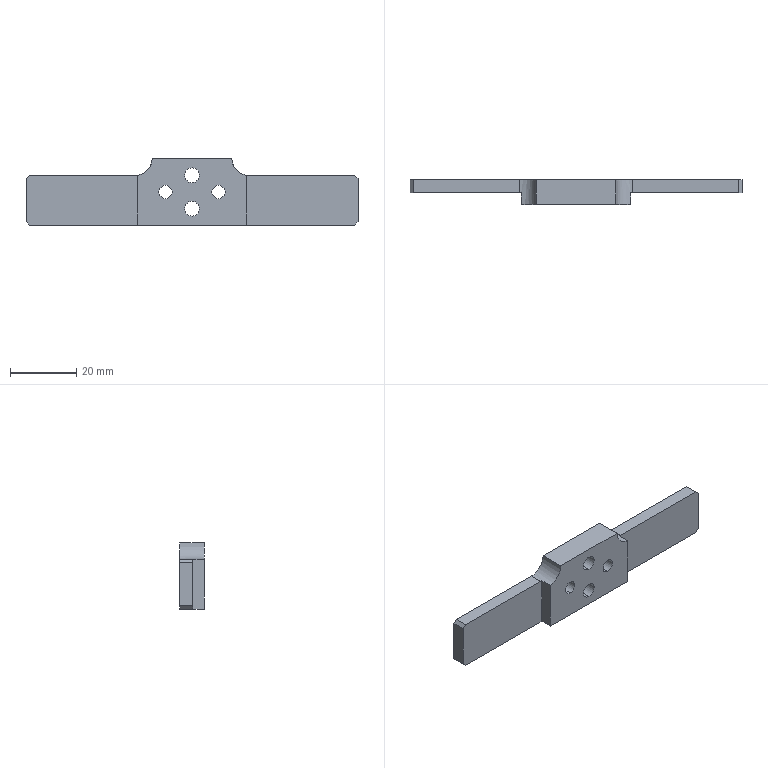Part | SolidWorks | features ICE 6, Chamfer 2, LPattern 2, Cut 1, Extrusion 1, Fillet 1, HoleWzd 1 | 1 solid | 26 faces | box 100 x 7.5 x 20 mm | volume 8278 mm3 | plane 16 | cylinder 10 | commonest cylinder face diameters 4 x4 4.5 x4 10 x2
STEP:
#1=CARTESIAN_POINT('',(-62.,-5.5,-7.));
#2=VERTEX_POINT('',#1);
#3=CARTESIAN_POINT('',(-62.,-5.5,-3.));
#4=VERTEX_POINT('',#3);
#5=CARTESIAN_POINT('',(-62.,-5.5,-5.));
#6=DIRECTION('',(0.,1.,0.));
#7=DIRECTION('',(0.,0.,1.));
#8=AXIS2_PLACEMENT_3D('',#5,#6,#7);
#9=CIRCLE('',#8,2.);
#10=EDGE_CURVE('',#2,#4,#9,.T.);
#11=ORIENTED_EDGE('',*,*,#10,.F.);
#12=CARTESIAN_POINT('',(-62.,2.,-7.));
#13=VERTEX_POINT('',#12);
#14=CARTESIAN_POINT('',(-62.,2.,-7.));
#15=DIRECTION('',(0.,1.,0.));
#16=VECTOR('',#15,1000.);
#17=LINE('',#14,#16);
#18=EDGE_CURVE('',#2,#13,#17,.T.);
#19=ORIENTED_EDGE('',*,*,#18,.T.);
#20=CARTESIAN_POINT('',(-62.,2.,-3.));
#21=VERTEX_POINT('',#20);
#22=CARTESIAN_POINT('',(-62.,2.,-5.));
#23=DIRECTION('',(0.,1.,0.));
#24=DIRECTION('',(0.,0.,1.));
#25=AXIS2_PLACEMENT_3D('',#22,#23,#24);
#26=CIRCLE('',#25,2.);
#27=EDGE_CURVE('',#13,#21,#26,.T.);
#28=ORIENTED_EDGE('',*,*,#27,.T.);
#29=CARTESIAN_POINT('',(-62.,2.,-3.));
#30=DIRECTION('',(0.,1.,0.));
#31=VECTOR('',#30,1000.);
#32=LINE('',#29,#31);
#33=EDGE_CURVE('',#4,#21,#32,.T.);
#34=ORIENTED_EDGE('',*,*,#33,.F.);
#35=EDGE_LOOP('',(#11,#19,#28,#34));
#36=FACE_OUTER_BOUND('',#35,.T.);
#37=CARTESIAN_POINT('',(-62.,2.,-5.));
#38=DIRECTION('',(0.,1.,0.));
#39=DIRECTION('',(0.,0.,1.));
#40=AXIS2_PLACEMENT_3D('',#37,#38,#39);
#41=CYLINDRICAL_SURFACE('',#40,2.);
#42=ADVANCED_FACE('',(#36),#41,.F.);
#43=CARTESIAN_POINT('',(-78.,-5.5,-7.));
#44=VERTEX_POINT('',#43);
#45=CARTESIAN_POINT('',(-78.,-5.5,-3.));
#46=VERTEX_POINT('',#45);
#47=CARTESIAN_POINT('',(-78.,-5.5,-5.));
#48=DIRECTION('',(0.,1.,0.));
#49=DIRECTION('',(0.,0.,1.));
#50=AXIS2_PLACEMENT_3D('',#47,#48,#49);
#51=CIRCLE('',#50,2.);
#52=EDGE_CURVE('',#44,#46,#51,.T.);
#53=ORIENTED_EDGE('',*,*,#52,.F.);
#54=CARTESIAN_POINT('',(-78.,2.,-7.));
#55=VERTEX_POINT('',#54);
#56=CARTESIAN_POINT('',(-78.,2.,-7.));
#57=DIRECTION('',(0.,1.,0.));
#58=VECTOR('',#57,1000.);
#59=LINE('',#56,#58);
#60=EDGE_CURVE('',#44,#55,#59,.T.);
#61=ORIENTED_EDGE('',*,*,#60,.T.);
#62=CARTESIAN_POINT('',(-78.,2.,-3.));
#63=VERTEX_POINT('',#62);
#64=CARTESIAN_POINT('',(-78.,2.,-5.));
#65=DIRECTION('',(0.,1.,0.));
#66=DIRECTION('',(0.,0.,1.));
#67=AXIS2_PLACEMENT_3D('',#64,#65,#66);
#68=CIRCLE('',#67,2.);
#69=EDGE_CURVE('',#55,#63,#68,.T.);
#70=ORIENTED_EDGE('',*,*,#69,.T.);
#71=CARTESIAN_POINT('',(-78.,2.,-3.));
#72=DIRECTION('',(0.,1.,0.));
#73=VECTOR('',#72,1000.);
#74=LINE('',#71,#73);
#75=EDGE_CURVE('',#46,#63,#74,.T.);
#76=ORIENTED_EDGE('',*,*,#75,.F.);
#77=EDGE_LOOP('',(#53,#61,#70,#76));
#78=FACE_OUTER_BOUND('',#77,.T.);
#79=CARTESIAN_POINT('',(-78.,2.,-5.));
#80=DIRECTION('',(0.,1.,0.));
#81=DIRECTION('',(0.,0.,1.));
#82=AXIS2_PLACEMENT_3D('',#79,#80,#81);
#83=CYLINDRICAL_SURFACE('',#82,2.);
#84=ADVANCED_FACE('',(#78),#83,.F.);
#85=CARTESIAN_POINT('',(-70.,-5.5,-7.75));
#86=VERTEX_POINT('',#85);
#87=CARTESIAN_POINT('',(-70.,-5.5,-12.25));
#88=VERTEX_POINT('',#87);
#89=CARTESIAN_POINT('',(-70.,-5.5,-10.));
#90=DIRECTION('',(0.,-1.,0.));
#91=DIRECTION('',(0.,0.,-1.));
#92=AXIS2_PLACEMENT_3D('',#89,#90,#91);
#93=CIRCLE('',#92,2.25);
#94=EDGE_CURVE('',#86,#88,#93,.T.);
#95=ORIENTED_EDGE('',*,*,#94,.T.);
#96=CARTESIAN_POINT('',(-70.,2.,-12.25));
#97=VERTEX_POINT('',#96);
#98=CARTESIAN_POINT('',(-70.,-5.5,-12.25));
#99=DIRECTION('',(0.,1.,0.));
#100=VECTOR('',#99,1000.);
#101=LINE('',#98,#100);
#102=EDGE_CURVE('',#88,#97,#101,.T.);
#103=ORIENTED_EDGE('',*,*,#102,.T.);
#104=CARTESIAN_POINT('',(-70.,2.,-7.75));
#105=VERTEX_POINT('',#104);
#106=CARTESIAN_POINT('',(-70.,2.,-10.));
#107=DIRECTION('',(0.,1.,0.));
#108=DIRECTION('',(0.,0.,1.));
#109=AXIS2_PLACEMENT_3D('',#106,#107,#108);
#110=CIRCLE('',#109,2.25);
#111=EDGE_CURVE('',#97,#105,#110,.T.);
#112=ORIENTED_EDGE('',*,*,#111,.T.);
#113=CARTESIAN_POINT('',(-70.,-5.5,-7.75));
#114=DIRECTION('',(0.,1.,0.));
#115=VECTOR('',#114,1000.);
#116=LINE('',#113,#115);
#117=EDGE_CURVE('',#86,#105,#116,.T.);
#118=ORIENTED_EDGE('',*,*,#117,.F.);
#119=EDGE_LOOP('',(#95,#103,#112,#118));
#120=FACE_OUTER_BOUND('',#119,.T.);
#121=CARTESIAN_POINT('',(-70.,-5.5,-10.));
#122=DIRECTION('',(0.,1.,0.));
#123=DIRECTION('',(0.,0.,1.));
#124=AXIS2_PLACEMENT_3D('',#121,#122,#123);
#125=CYLINDRICAL_SURFACE('',#124,2.25);
#126=ADVANCED_FACE('',(#120),#125,.F.);
#127=CARTESIAN_POINT('',(-70.,-5.5,2.25));
#128=VERTEX_POINT('',#127);
#129=CARTESIAN_POINT('',(-70.,-5.5,-2.25));
#130=VERTEX_POINT('',#129);
#131=CARTESIAN_POINT('',(-70.,-5.5,0.));
#132=DIRECTION('',(0.,-1.,0.));
#133=DIRECTION('',(0.,0.,-1.));
#134=AXIS2_PLACEMENT_3D('',#131,#132,#133);
#135=CIRCLE('',#134,2.25);
#136=EDGE_CURVE('',#128,#130,#135,.T.);
#137=ORIENTED_EDGE('',*,*,#136,.T.);
#138=CARTESIAN_POINT('',(-70.,2.,-2.25));
#139=VERTEX_POINT('',#138);
#140=CARTESIAN_POINT('',(-70.,-5.5,-2.25));
#141=DIRECTION('',(0.,1.,0.));
#142=VECTOR('',#141,1000.);
#143=LINE('',#140,#142);
#144=EDGE_CURVE('',#130,#139,#143,.T.);
#145=ORIENTED_EDGE('',*,*,#144,.T.);
#146=CARTESIAN_POINT('',(-70.,2.,2.25));
#147=VERTEX_POINT('',#146);
#148=CARTESIAN_POINT('',(-70.,2.,0.));
#149=DIRECTION('',(0.,1.,0.));
#150=DIRECTION('',(0.,0.,1.));
#151=AXIS2_PLACEMENT_3D('',#148,#149,#150);
#152=CIRCLE('',#151,2.25);
#153=EDGE_CURVE('',#139,#147,#152,.T.);
#154=ORIENTED_EDGE('',*,*,#153,.T.);
#155=CARTESIAN_POINT('',(-70.,-5.5,2.25));
#156=DIRECTION('',(0.,1.,0.));
#157=VECTOR('',#156,1000.);
#158=LINE('',#155,#157);
#159=EDGE_CURVE('',#128,#147,#158,.T.);
#160=ORIENTED_EDGE('',*,*,#159,.F.);
#161=EDGE_LOOP('',(#137,#145,#154,#160));
#162=FACE_OUTER_BOUND('',#161,.T.);
#163=CARTESIAN_POINT('',(-70.,-5.5,0.));
#164=DIRECTION('',(0.,1.,0.));
#165=DIRECTION('',(0.,0.,1.));
#166=AXIS2_PLACEMENT_3D('',#163,#164,#165);
#167=CYLINDRICAL_SURFACE('',#166,2.25);
#168=ADVANCED_FACE('',(#162),#167,.F.);
#169=CARTESIAN_POINT('',(-119.,-2.,-15.));
#170=VERTEX_POINT('',#169);
#171=CARTESIAN_POINT('',(-86.5,-2.,-15.));
#172=VERTEX_POINT('',#171);
#173=CARTESIAN_POINT('',(-69.,-2.,-15.));
#174=DIRECTION('',(1.,0.,0.));
#175=VECTOR('',#174,1000.);
#176=LINE('',#173,#175);
#177=EDGE_CURVE('',#170,#172,#176,.T.);
#178=ORIENTED_EDGE('',*,*,#177,.T.);
#179=CARTESIAN_POINT('',(-86.5,-2.,0.02506));
#180=VERTEX_POINT('',#179);
#181=CARTESIAN_POINT('',(-86.5,-2.,-15.));
#182=DIRECTION('',(0.,0.,-1.));
#183=VECTOR('',#182,1000.);
#184=LINE('',#181,#183);
#185=EDGE_CURVE('',#180,#172,#184,.T.);
#186=ORIENTED_EDGE('',*,*,#185,.F.);
#187=CARTESIAN_POINT('',(-87.,-2.,0.));
#188=VERTEX_POINT('',#187);
#189=CARTESIAN_POINT('',(-87.,-2.,5.));
#190=DIRECTION('',(0.,1.,0.));
#191=DIRECTION('',(0.,0.,1.));
#192=AXIS2_PLACEMENT_3D('',#189,#190,#191);
#193=CIRCLE('',#192,5.);
#194=EDGE_CURVE('',#180,#188,#193,.T.);
#195=ORIENTED_EDGE('',*,*,#194,.T.);
#196=CARTESIAN_POINT('',(-119.,-2.,0.));
#197=VERTEX_POINT('',#196);
#198=CARTESIAN_POINT('',(-120.,-2.,0.));
#199=DIRECTION('',(1.,0.,0.));
#200=VECTOR('',#199,1000.);
#201=LINE('',#198,#200);
#202=EDGE_CURVE('',#197,#188,#201,.T.);
#203=ORIENTED_EDGE('',*,*,#202,.F.);
#204=CARTESIAN_POINT('',(-120.,-2.,-1.));
#205=VERTEX_POINT('',#204);
#206=CARTESIAN_POINT('',(-120.,-2.,-1.));
#207=DIRECTION('',(-0.7071,0.,-0.7071));
#208=VECTOR('',#207,1000.);
#209=LINE('',#206,#208);
#210=EDGE_CURVE('',#197,#205,#209,.T.);
#211=ORIENTED_EDGE('',*,*,#210,.T.);
#212=CARTESIAN_POINT('',(-120.,-2.,-14.));
#213=VERTEX_POINT('',#212);
#214=CARTESIAN_POINT('',(-120.,-2.,-15.));
#215=DIRECTION('',(0.,0.,1.));
#216=VECTOR('',#215,1000.);
#217=LINE('',#214,#216);
#218=EDGE_CURVE('',#213,#205,#217,.T.);
#219=ORIENTED_EDGE('',*,*,#218,.F.);
#220=CARTESIAN_POINT('',(-119.,-2.,-15.));
#221=DIRECTION('',(0.7071,0.,-0.7071));
#222=VECTOR('',#221,1000.);
#223=LINE('',#220,#222);
#224=EDGE_CURVE('',#213,#170,#223,.T.);
#225=ORIENTED_EDGE('',*,*,#224,.T.);
#226=EDGE_LOOP('',(#178,#186,#195,#203,#211,#219,#225));
#227=FACE_OUTER_BOUND('',#226,.T.);
#228=CARTESIAN_POINT('',(-53.,-2.,5.));
#229=DIRECTION('',(0.,1.,0.));
#230=DIRECTION('',(0.,0.,1.));
#231=AXIS2_PLACEMENT_3D('',#228,#229,#230);
#232=PLANE('',#231);
#233=ADVANCED_FACE('',(#227),#232,.F.);
#234=CARTESIAN_POINT('',(-53.,-2.,0.));
#235=VERTEX_POINT('',#234);
#236=CARTESIAN_POINT('',(-53.5,-2.,0.02506));
#237=VERTEX_POINT('',#236);
#238=CARTESIAN_POINT('',(-53.,-2.,5.));
#239=DIRECTION('',(0.,1.,0.));
#240=DIRECTION('',(0.,0.,1.));
#241=AXIS2_PLACEMENT_3D('',#238,#239,#240);
#242=CIRCLE('',#241,5.);
#243=EDGE_CURVE('',#235,#237,#242,.T.);
#244=ORIENTED_EDGE('',*,*,#243,.T.);
#245=CARTESIAN_POINT('',(-53.5,-2.,-15.));
#246=VERTEX_POINT('',#245);
#247=CARTESIAN_POINT('',(-53.5,-2.,-15.));
#248=DIRECTION('',(0.,0.,1.));
#249=VECTOR('',#248,1000.);
#250=LINE('',#247,#249);
#251=EDGE_CURVE('',#246,#237,#250,.T.);
#252=ORIENTED_EDGE('',*,*,#251,.F.);
#253=CARTESIAN_POINT('',(-21.,-2.,-15.));
#254=VERTEX_POINT('',#253);
#255=CARTESIAN_POINT('',(-69.,-2.,-15.));
#256=DIRECTION('',(1.,0.,0.));
#257=VECTOR('',#256,1000.);
#258=LINE('',#255,#257);
#259=EDGE_CURVE('',#246,#254,#258,.T.);
#260=ORIENTED_EDGE('',*,*,#259,.T.);
#261=CARTESIAN_POINT('',(-20.,-2.,-14.));
#262=VERTEX_POINT('',#261);
#263=CARTESIAN_POINT('',(-20.,-2.,-14.));
#264=DIRECTION('',(0.7071,0.,0.7071));
#265=VECTOR('',#264,1000.);
#266=LINE('',#263,#265);
#267=EDGE_CURVE('',#254,#262,#266,.T.);
#268=ORIENTED_EDGE('',*,*,#267,.T.);
#269=CARTESIAN_POINT('',(-20.,-2.,-1.));
#270=VERTEX_POINT('',#269);
#271=CARTESIAN_POINT('',(-20.,-2.,5.));
#272=DIRECTION('',(0.,0.,1.));
#273=VECTOR('',#272,1000.);
#274=LINE('',#271,#273);
#275=EDGE_CURVE('',#262,#270,#274,.T.);
#276=ORIENTED_EDGE('',*,*,#275,.T.);
#277=CARTESIAN_POINT('',(-21.,-2.,0.));
#278=VERTEX_POINT('',#277);
#279=CARTESIAN_POINT('',(-20.,-2.,-1.));
#280=DIRECTION('',(-0.7071,0.,0.7071));
#281=VECTOR('',#280,1000.);
#282=LINE('',#279,#281);
#283=EDGE_CURVE('',#270,#278,#282,.T.);
#284=ORIENTED_EDGE('',*,*,#283,.T.);
#285=CARTESIAN_POINT('',(69.,-2.,0.));
#286=DIRECTION('',(-1.,0.,0.));
#287=VECTOR('',#286,1000.);
#288=LINE('',#285,#287);
#289=EDGE_CURVE('',#278,#235,#288,.T.);
#290=ORIENTED_EDGE('',*,*,#289,.T.);
#291=EDGE_LOOP('',(#244,#252,#260,#268,#276,#284,#290));
#292=FACE_OUTER_BOUND('',#291,.T.);
#293=CARTESIAN_POINT('',(-53.,-2.,5.));
#294=DIRECTION('',(0.,1.,0.));
#295=DIRECTION('',(0.,0.,1.));
#296=AXIS2_PLACEMENT_3D('',#293,#294,#295);
#297=PLANE('',#296);
#298=ADVANCED_FACE('',(#292),#297,.F.);
#299=ORIENTED_EDGE('',*,*,#243,.F.);
#300=CARTESIAN_POINT('',(-53.,2.,0.));
#301=VERTEX_POINT('',#300);
#302=CARTESIAN_POINT('',(-53.,2.,0.));
#303=DIRECTION('',(0.,-1.,0.));
#304=VECTOR('',#303,1000.);
#305=LINE('',#302,#304);
#306=EDGE_CURVE('',#301,#235,#305,.T.);
#307=ORIENTED_EDGE('',*,*,#306,.F.);
#308=CARTESIAN_POINT('',(-58.,2.,5.));
#309=VERTEX_POINT('',#308);
#310=CARTESIAN_POINT('',(-53.,2.,5.));
#311=DIRECTION('',(0.,1.,0.));
#312=DIRECTION('',(0.,0.,1.));
#313=AXIS2_PLACEMENT_3D('',#310,#311,#312);
#314=CIRCLE('',#313,5.);
#315=EDGE_CURVE('',#301,#309,#314,.T.);
#316=ORIENTED_EDGE('',*,*,#315,.T.);
#317=CARTESIAN_POINT('',(-58.,-5.5,5.));
#318=VERTEX_POINT('',#317);
#319=CARTESIAN_POINT('',(-58.,2.,5.));
#320=DIRECTION('',(0.,-1.,0.));
#321=VECTOR('',#320,1000.);
#322=LINE('',#319,#321);
#323=EDGE_CURVE('',#309,#318,#322,.T.);
#324=ORIENTED_EDGE('',*,*,#323,.T.);
#325=CARTESIAN_POINT('',(-53.5,-5.5,0.02506));
#326=VERTEX_POINT('',#325);
#327=CARTESIAN_POINT('',(-53.,-5.5,5.));
#328=DIRECTION('',(0.,-1.,0.));
#329=DIRECTION('',(0.,0.,-1.));
#330=AXIS2_PLACEMENT_3D('',#327,#328,#329);
#331=CIRCLE('',#330,5.);
#332=EDGE_CURVE('',#318,#326,#331,.T.);
#333=ORIENTED_EDGE('',*,*,#332,.T.);
#334=CARTESIAN_POINT('',(-53.5,-6.,0.02506));
#335=DIRECTION('',(0.,1.,0.));
#336=VECTOR('',#335,1000.);
#337=LINE('',#334,#336);
#338=EDGE_CURVE('',#326,#237,#337,.T.);
#339=ORIENTED_EDGE('',*,*,#338,.T.);
#340=EDGE_LOOP('',(#299,#307,#316,#324,#333,#339));
#341=FACE_OUTER_BOUND('',#340,.T.);
#342=CARTESIAN_POINT('',(-53.,2.,5.));
#343=DIRECTION('',(0.,-1.,0.));
#344=DIRECTION('',(0.,0.,-1.));
#345=AXIS2_PLACEMENT_3D('',#342,#343,#344);
#346=CYLINDRICAL_SURFACE('',#345,5.);
#347=ADVANCED_FACE('',(#341),#346,.F.);
#348=ORIENTED_EDGE('',*,*,#289,.F.);
#349=CARTESIAN_POINT('',(-21.,2.,0.));
#350=VERTEX_POINT('',#349);
#351=CARTESIAN_POINT('',(-21.,2.,0.));
#352=DIRECTION('',(0.,1.,0.));
#353=VECTOR('',#352,1000.);
#354=LINE('',#351,#353);
#355=EDGE_CURVE('',#278,#350,#354,.T.);
#356=ORIENTED_EDGE('',*,*,#355,.T.);
#357=CARTESIAN_POINT('',(69.,2.,0.));
#358=DIRECTION('',(-1.,0.,0.));
#359=VECTOR('',#358,1000.);
#360=LINE('',#357,#359);
#361=EDGE_CURVE('',#350,#301,#360,.T.);
#362=ORIENTED_EDGE('',*,*,#361,.T.);
#363=ORIENTED_EDGE('',*,*,#306,.T.);
#364=EDGE_LOOP('',(#348,#356,#362,#363));
#365=FACE_OUTER_BOUND('',#364,.T.);
#366=CARTESIAN_POINT('',(69.,2.,0.));
#367=DIRECTION('',(0.,0.,1.));
#368=DIRECTION('',(1.,0.,0.));
#369=AXIS2_PLACEMENT_3D('',#366,#367,#368);
#370=PLANE('',#369);
#371=ADVANCED_FACE('',(#365),#370,.T.);
#372=ORIENTED_EDGE('',*,*,#259,.F.);
#373=CARTESIAN_POINT('',(-53.5,-5.5,-15.));
#374=VERTEX_POINT('',#373);
#375=CARTESIAN_POINT('',(-53.5,18.5,-15.));
#376=DIRECTION('',(0.,-1.,0.));
#377=VECTOR('',#376,1000.);
#378=LINE('',#375,#377);
#379=EDGE_CURVE('',#246,#374,#378,.T.);
#380=ORIENTED_EDGE('',*,*,#379,.T.);
#381=CARTESIAN_POINT('',(-86.5,-5.5,-15.));
#382=VERTEX_POINT('',#381);
#383=CARTESIAN_POINT('',(-82.,-5.5,-15.));
#384=DIRECTION('',(1.,0.,0.));
#385=VECTOR('',#384,1000.);
#386=LINE('',#383,#385);
#387=EDGE_CURVE('',#382,#374,#386,.T.);
#388=ORIENTED_EDGE('',*,*,#387,.F.);
#389=CARTESIAN_POINT('',(-86.5,18.5,-15.));
#390=DIRECTION('',(0.,-1.,0.));
#391=VECTOR('',#390,1000.);
#392=LINE('',#389,#391);
#393=EDGE_CURVE('',#172,#382,#392,.T.);
#394=ORIENTED_EDGE('',*,*,#393,.F.);
#395=ORIENTED_EDGE('',*,*,#177,.F.);
#396=CARTESIAN_POINT('',(-119.,2.,-15.));
#397=VERTEX_POINT('',#396);
#398=CARTESIAN_POINT('',(-119.,2.,-15.));
#399=DIRECTION('',(0.,1.,0.));
#400=VECTOR('',#399,1000.);
#401=LINE('',#398,#400);
#402=EDGE_CURVE('',#170,#397,#401,.T.);
#403=ORIENTED_EDGE('',*,*,#402,.T.);
#404=CARTESIAN_POINT('',(-21.,2.,-15.));
#405=VERTEX_POINT('',#404);
#406=CARTESIAN_POINT('',(-69.,2.,-15.));
#407=DIRECTION('',(1.,0.,0.));
#408=VECTOR('',#407,1000.);
#409=LINE('',#406,#408);
#410=EDGE_CURVE('',#397,#405,#409,.T.);
#411=ORIENTED_EDGE('',*,*,#410,.T.);
#412=CARTESIAN_POINT('',(-21.,-2.,-15.));
#413=DIRECTION('',(0.,-1.,0.));
#414=VECTOR('',#413,1000.);
#415=LINE('',#412,#414);
#416=EDGE_CURVE('',#405,#254,#415,.T.);
#417=ORIENTED_EDGE('',*,*,#416,.T.);
#418=EDGE_LOOP('',(#372,#380,#388,#394,#395,#403,#411,#417));
#419=FACE_OUTER_BOUND('',#418,.T.);
#420=CARTESIAN_POINT('',(-69.,2.,-15.));
#421=DIRECTION('',(0.,0.,-1.));
#422=DIRECTION('',(-1.,0.,0.));
#423=AXIS2_PLACEMENT_3D('',#420,#421,#422);
#424=PLANE('',#423);
#425=ADVANCED_FACE('',(#419),#424,.T.);
#426=CARTESIAN_POINT('',(-62.,2.,-5.));
#427=DIRECTION('',(0.,1.,0.));
#428=DIRECTION('',(0.,0.,1.));
#429=AXIS2_PLACEMENT_3D('',#426,#427,#428);
#430=CIRCLE('',#429,2.);
#431=EDGE_CURVE('',#21,#13,#430,.T.);
#432=ORIENTED_EDGE('',*,*,#431,.F.);
#433=ORIENTED_EDGE('',*,*,#27,.F.);
#434=EDGE_LOOP('',(#432,#433));
#435=FACE_BOUND('',#434,.T.);
#436=CARTESIAN_POINT('',(-78.,2.,-5.));
#437=DIRECTION('',(0.,1.,0.));
#438=DIRECTION('',(0.,0.,1.));
#439=AXIS2_PLACEMENT_3D('',#436,#437,#438);
#440=CIRCLE('',#439,2.);
#441=EDGE_CURVE('',#63,#55,#440,.T.);
#442=ORIENTED_EDGE('',*,*,#441,.F.);
#443=ORIENTED_EDGE('',*,*,#69,.F.);
#444=EDGE_LOOP('',(#442,#443));
#445=FACE_BOUND('',#444,.T.);
#446=ORIENTED_EDGE('',*,*,#361,.F.);
#447=CARTESIAN_POINT('',(-20.,2.,-1.));
#448=VERTEX_POINT('',#447);
#449=CARTESIAN_POINT('',(-39.5,2.,18.5));
#450=DIRECTION('',(0.7071,0.,-0.7071));
#451=VECTOR('',#450,1000.);
#452=LINE('',#449,#451);
#453=EDGE_CURVE('',#350,#448,#452,.T.);
#454=ORIENTED_EDGE('',*,*,#453,.T.);
#455=CARTESIAN_POINT('',(-20.,2.,-14.));
#456=VERTEX_POINT('',#455);
#457=CARTESIAN_POINT('',(-20.,2.,5.));
#458=DIRECTION('',(0.,0.,1.));
#459=VECTOR('',#458,1000.);
#460=LINE('',#457,#459);
#461=EDGE_CURVE('',#456,#448,#460,.T.);
#462=ORIENTED_EDGE('',*,*,#461,.F.);
#463=CARTESIAN_POINT('',(-27.,2.,-21.));
#464=DIRECTION('',(-0.7071,0.,-0.7071));
#465=VECTOR('',#464,1000.);
#466=LINE('',#463,#465);
#467=EDGE_CURVE('',#456,#405,#466,.T.);
#468=ORIENTED_EDGE('',*,*,#467,.T.);
#469=ORIENTED_EDGE('',*,*,#410,.F.);
#470=CARTESIAN_POINT('',(-120.,2.,-14.));
#471=VERTEX_POINT('',#470);
#472=CARTESIAN_POINT('',(-96.,2.,-38.));
#473=DIRECTION('',(-0.7071,0.,0.7071));
#474=VECTOR('',#473,1000.);
#475=LINE('',#472,#474);
#476=EDGE_CURVE('',#397,#471,#475,.T.);
#477=ORIENTED_EDGE('',*,*,#476,.T.);
#478=CARTESIAN_POINT('',(-120.,2.,-1.));
#479=VERTEX_POINT('',#478);
#480=CARTESIAN_POINT('',(-120.,2.,-15.));
#481=DIRECTION('',(0.,0.,1.));
#482=VECTOR('',#481,1000.);
#483=LINE('',#480,#482);
#484=EDGE_CURVE('',#471,#479,#483,.T.);
#485=ORIENTED_EDGE('',*,*,#484,.T.);
#486=CARTESIAN_POINT('',(-119.,2.,0.));
#487=VERTEX_POINT('',#486);
#488=CARTESIAN_POINT('',(-83.5,2.,35.5));
#489=DIRECTION('',(0.7071,0.,0.7071));
#490=VECTOR('',#489,1000.);
#491=LINE('',#488,#490);
#492=EDGE_CURVE('',#479,#487,#491,.T.);
#493=ORIENTED_EDGE('',*,*,#492,.T.);
#494=CARTESIAN_POINT('',(-87.,2.,0.));
#495=VERTEX_POINT('',#494);
#496=CARTESIAN_POINT('',(-120.,2.,0.));
#497=DIRECTION('',(1.,0.,0.));
#498=VECTOR('',#497,1000.);
#499=LINE('',#496,#498);
#500=EDGE_CURVE('',#487,#495,#499,.T.);
#501=ORIENTED_EDGE('',*,*,#500,.T.);
#502=CARTESIAN_POINT('',(-82.,2.,5.));
#503=VERTEX_POINT('',#502);
#504=CARTESIAN_POINT('',(-87.,2.,5.));
#505=DIRECTION('',(0.,-1.,0.));
#506=DIRECTION('',(0.,0.,1.));
#507=AXIS2_PLACEMENT_3D('',#504,#505,#506);
#508=CIRCLE('',#507,5.);
#509=EDGE_CURVE('',#495,#503,#508,.T.);
#510=ORIENTED_EDGE('',*,*,#509,.T.);
#511=CARTESIAN_POINT('',(-58.,2.,5.));
#512=DIRECTION('',(-1.,0.,0.));
#513=VECTOR('',#512,1000.);
#514=LINE('',#511,#513);
#515=EDGE_CURVE('',#309,#503,#514,.T.);
#516=ORIENTED_EDGE('',*,*,#515,.F.);
#517=ORIENTED_EDGE('',*,*,#315,.F.);
#518=EDGE_LOOP('',(#446,#454,#462,#468,#469,#477,#485,#493,#501,#510,#516,#517));
#519=FACE_OUTER_BOUND('',#518,.T.);
#520=CARTESIAN_POINT('',(-70.,2.,0.));
#521=DIRECTION('',(0.,1.,0.));
#522=DIRECTION('',(0.,0.,1.));
#523=AXIS2_PLACEMENT_3D('',#520,#521,#522);
#524=CIRCLE('',#523,2.25);
#525=EDGE_CURVE('',#147,#139,#524,.T.);
#526=ORIENTED_EDGE('',*,*,#525,.F.);
#527=ORIENTED_EDGE('',*,*,#153,.F.);
#528=EDGE_LOOP('',(#526,#527));
#529=FACE_BOUND('',#528,.T.);
#530=CARTESIAN_POINT('',(-70.,2.,-10.));
#531=DIRECTION('',(0.,1.,0.));
#532=DIRECTION('',(0.,0.,1.));
#533=AXIS2_PLACEMENT_3D('',#530,#531,#532);
#534=CIRCLE('',#533,2.25);
#535=EDGE_CURVE('',#105,#97,#534,.T.);
#536=ORIENTED_EDGE('',*,*,#535,.F.);
#537=ORIENTED_EDGE('',*,*,#111,.F.);
#538=EDGE_LOOP('',(#536,#537));
#539=FACE_BOUND('',#538,.T.);
#540=CARTESIAN_POINT('',(-53.,2.,5.));
#541=DIRECTION('',(0.,1.,0.));
#542=DIRECTION('',(0.,0.,1.));
#543=AXIS2_PLACEMENT_3D('',#540,#541,#542);
#544=PLANE('',#543);
#545=ADVANCED_FACE('',(#435,#445,#519,#529,#539),#544,.T.);
#546=ORIENTED_EDGE('',*,*,#500,.F.);
#547=CARTESIAN_POINT('',(-119.,-2.,0.));
#548=DIRECTION('',(0.,-1.,0.));
#549=VECTOR('',#548,1000.);
#550=LINE('',#547,#549);
#551=EDGE_CURVE('',#487,#197,#550,.T.);
#552=ORIENTED_EDGE('',*,*,#551,.T.);
#553=ORIENTED_EDGE('',*,*,#202,.T.);
#554=CARTESIAN_POINT('',(-87.,2.,0.));
#555=DIRECTION('',(0.,1.,0.));
#556=VECTOR('',#555,1000.);
#557=LINE('',#554,#556);
#558=EDGE_CURVE('',#188,#495,#557,.T.);
#559=ORIENTED_EDGE('',*,*,#558,.T.);
#560=EDGE_LOOP('',(#546,#552,#553,#559));
#561=FACE_OUTER_BOUND('',#560,.T.);
#562=CARTESIAN_POINT('',(-120.,-2.,0.));
#563=DIRECTION('',(0.,0.,1.));
#564=DIRECTION('',(1.,0.,0.));
#565=AXIS2_PLACEMENT_3D('',#562,#563,#564);
#566=PLANE('',#565);
#567=ADVANCED_FACE('',(#561),#566,.T.);
#568=ORIENTED_EDGE('',*,*,#218,.T.);
#569=CARTESIAN_POINT('',(-120.,-2.,-1.));
#570=DIRECTION('',(0.,1.,0.));
#571=VECTOR('',#570,1000.);
#572=LINE('',#569,#571);
#573=EDGE_CURVE('',#205,#479,#572,.T.);
#574=ORIENTED_EDGE('',*,*,#573,.T.);
#575=ORIENTED_EDGE('',*,*,#484,.F.);
#576=CARTESIAN_POINT('',(-120.,-2.,-14.));
#577=DIRECTION('',(0.,-1.,0.));
#578=VECTOR('',#577,1000.);
#579=LINE('',#576,#578);
#580=EDGE_CURVE('',#471,#213,#579,.T.);
#581=ORIENTED_EDGE('',*,*,#580,.T.);
#582=EDGE_LOOP('',(#568,#574,#575,#581));
#583=FACE_OUTER_BOUND('',#582,.T.);
#584=CARTESIAN_POINT('',(-120.,-2.,-15.));
#585=DIRECTION('',(-1.,0.,0.));
#586=DIRECTION('',(0.,0.,1.));
#587=AXIS2_PLACEMENT_3D('',#584,#585,#586);
#588=PLANE('',#587);
#589=ADVANCED_FACE('',(#583),#588,.T.);
#590=ORIENTED_EDGE('',*,*,#194,.F.);
#591=CARTESIAN_POINT('',(-86.5,-5.5,0.02506));
#592=VERTEX_POINT('',#591);
#593=CARTESIAN_POINT('',(-86.5,-6.,0.02506));
#594=DIRECTION('',(0.,-1.,0.));
#595=VECTOR('',#594,1000.);
#596=LINE('',#593,#595);
#597=EDGE_CURVE('',#180,#592,#596,.T.);
#598=ORIENTED_EDGE('',*,*,#597,.T.);
#599=CARTESIAN_POINT('',(-82.,-5.5,5.));
#600=VERTEX_POINT('',#599);
#601=CARTESIAN_POINT('',(-87.,-5.5,5.));
#602=DIRECTION('',(0.,-1.,0.));
#603=DIRECTION('',(0.,0.,-1.));
#604=AXIS2_PLACEMENT_3D('',#601,#602,#603);
#605=CIRCLE('',#604,5.);
#606=EDGE_CURVE('',#592,#600,#605,.T.);
#607=ORIENTED_EDGE('',*,*,#606,.T.);
#608=CARTESIAN_POINT('',(-82.,-2.,5.));
#609=DIRECTION('',(0.,-1.,0.));
#610=VECTOR('',#609,1000.);
#611=LINE('',#608,#610);
#612=EDGE_CURVE('',#503,#600,#611,.T.);
#613=ORIENTED_EDGE('',*,*,#612,.F.);
#614=ORIENTED_EDGE('',*,*,#509,.F.);
#615=ORIENTED_EDGE('',*,*,#558,.F.);
#616=EDGE_LOOP('',(#590,#598,#607,#613,#614,#615));
#617=FACE_OUTER_BOUND('',#616,.T.);
#618=CARTESIAN_POINT('',(-87.,-2.,5.));
#619=DIRECTION('',(0.,-1.,0.));
#620=DIRECTION('',(0.,0.,-1.));
#621=AXIS2_PLACEMENT_3D('',#618,#619,#620);
#622=CYLINDRICAL_SURFACE('',#621,5.);
#623=ADVANCED_FACE('',(#617),#622,.F.);
#624=CARTESIAN_POINT('',(-62.,-5.5,-5.));
#625=DIRECTION('',(0.,1.,0.));
#626=DIRECTION('',(0.,0.,1.));
#627=AXIS2_PLACEMENT_3D('',#624,#625,#626);
#628=CIRCLE('',#627,2.);
#629=EDGE_CURVE('',#4,#2,#628,.T.);
#630=ORIENTED_EDGE('',*,*,#629,.T.);
#631=ORIENTED_EDGE('',*,*,#10,.T.);
#632=EDGE_LOOP('',(#630,#631));
#633=FACE_BOUND('',#632,.T.);
#634=CARTESIAN_POINT('',(-78.,-5.5,-5.));
#635=DIRECTION('',(0.,1.,0.));
#636=DIRECTION('',(0.,0.,1.));
#637=AXIS2_PLACEMENT_3D('',#634,#635,#636);
#638=CIRCLE('',#637,2.);
#639=EDGE_CURVE('',#46,#44,#638,.T.);
#640=ORIENTED_EDGE('',*,*,#639,.T.);
#641=ORIENTED_EDGE('',*,*,#52,.T.);
#642=EDGE_LOOP('',(#640,#641));
#643=FACE_BOUND('',#642,.T.);
#644=ORIENTED_EDGE('',*,*,#332,.F.);
#645=CARTESIAN_POINT('',(-82.,-5.5,5.));
#646=DIRECTION('',(1.,0.,0.));
#647=VECTOR('',#646,1000.);
#648=LINE('',#645,#647);
#649=EDGE_CURVE('',#600,#318,#648,.T.);
#650=ORIENTED_EDGE('',*,*,#649,.F.);
#651=ORIENTED_EDGE('',*,*,#606,.F.);
#652=CARTESIAN_POINT('',(-86.5,-5.5,-15.));
#653=DIRECTION('',(0.,0.,-1.));
#654=VECTOR('',#653,1000.);
#655=LINE('',#652,#654);
#656=EDGE_CURVE('',#592,#382,#655,.T.);
#657=ORIENTED_EDGE('',*,*,#656,.T.);
#658=ORIENTED_EDGE('',*,*,#387,.T.);
#659=CARTESIAN_POINT('',(-53.5,-5.5,-15.));
#660=DIRECTION('',(0.,0.,1.));
#661=VECTOR('',#660,1000.);
#662=LINE('',#659,#661);
#663=EDGE_CURVE('',#374,#326,#662,.T.);
#664=ORIENTED_EDGE('',*,*,#663,.T.);
#665=EDGE_LOOP('',(#644,#650,#651,#657,#658,#664));
#666=FACE_OUTER_BOUND('',#665,.T.);
#667=ORIENTED_EDGE('',*,*,#136,.F.);
#668=CARTESIAN_POINT('',(-70.,-5.5,0.));
#669=DIRECTION('',(0.,-1.,0.));
#670=DIRECTION('',(0.,0.,-1.));
#671=AXIS2_PLACEMENT_3D('',#668,#669,#670);
#672=CIRCLE('',#671,2.25);
#673=EDGE_CURVE('',#130,#128,#672,.T.);
#674=ORIENTED_EDGE('',*,*,#673,.F.);
#675=EDGE_LOOP('',(#667,#674));
#676=FACE_BOUND('',#675,.T.);
#677=ORIENTED_EDGE('',*,*,#94,.F.);
#678=CARTESIAN_POINT('',(-70.,-5.5,-10.));
#679=DIRECTION('',(0.,-1.,0.));
#680=DIRECTION('',(0.,0.,-1.));
#681=AXIS2_PLACEMENT_3D('',#678,#679,#680);
#682=CIRCLE('',#681,2.25);
#683=EDGE_CURVE('',#88,#86,#682,.T.);
#684=ORIENTED_EDGE('',*,*,#683,.F.);
#685=EDGE_LOOP('',(#677,#684));
#686=FACE_BOUND('',#685,.T.);
#687=CARTESIAN_POINT('',(-82.,-5.5,-15.));
#688=DIRECTION('',(0.,-1.,0.));
#689=DIRECTION('',(0.,0.,-1.));
#690=AXIS2_PLACEMENT_3D('',#687,#688,#689);
#691=PLANE('',#690);
#692=ADVANCED_FACE('',(#633,#643,#666,#676,#686),#691,.T.);
#693=ORIENTED_EDGE('',*,*,#144,.F.);
#694=ORIENTED_EDGE('',*,*,#673,.T.);
#695=ORIENTED_EDGE('',*,*,#159,.T.);
#696=ORIENTED_EDGE('',*,*,#525,.T.);
#697=EDGE_LOOP('',(#693,#694,#695,#696));
#698=FACE_OUTER_BOUND('',#697,.T.);
#699=CARTESIAN_POINT('',(-70.,-5.5,0.));
#700=DIRECTION('',(0.,1.,0.));
#701=DIRECTION('',(0.,0.,1.));
#702=AXIS2_PLACEMENT_3D('',#699,#700,#701);
#703=CYLINDRICAL_SURFACE('',#702,2.25);
#704=ADVANCED_FACE('',(#698),#703,.F.);
#705=ORIENTED_EDGE('',*,*,#102,.F.);
#706=ORIENTED_EDGE('',*,*,#683,.T.);
#707=ORIENTED_EDGE('',*,*,#117,.T.);
#708=ORIENTED_EDGE('',*,*,#535,.T.);
#709=EDGE_LOOP('',(#705,#706,#707,#708));
#710=FACE_OUTER_BOUND('',#709,.T.);
#711=CARTESIAN_POINT('',(-70.,-5.5,-10.));
#712=DIRECTION('',(0.,1.,0.));
#713=DIRECTION('',(0.,0.,1.));
#714=AXIS2_PLACEMENT_3D('',#711,#712,#713);
#715=CYLINDRICAL_SURFACE('',#714,2.25);
#716=ADVANCED_FACE('',(#710),#715,.F.);
#717=ORIENTED_EDGE('',*,*,#461,.T.);
#718=CARTESIAN_POINT('',(-20.,-2.,-1.));
#719=DIRECTION('',(0.,-1.,0.));
#720=VECTOR('',#719,1000.);
#721=LINE('',#718,#720);
#722=EDGE_CURVE('',#448,#270,#721,.T.);
#723=ORIENTED_EDGE('',*,*,#722,.T.);
#724=ORIENTED_EDGE('',*,*,#275,.F.);
#725=CARTESIAN_POINT('',(-20.,2.,-14.));
#726=DIRECTION('',(0.,1.,0.));
#727=VECTOR('',#726,1000.);
#728=LINE('',#725,#727);
#729=EDGE_CURVE('',#262,#456,#728,.T.);
#730=ORIENTED_EDGE('',*,*,#729,.T.);
#731=EDGE_LOOP('',(#717,#723,#724,#730));
#732=FACE_OUTER_BOUND('',#731,.T.);
#733=CARTESIAN_POINT('',(-20.,-8.,21.15));
#734=DIRECTION('',(-1.,0.,0.));
#735=DIRECTION('',(0.,0.,1.));
#736=AXIS2_PLACEMENT_3D('',#733,#734,#735);
#737=PLANE('',#736);
#738=ADVANCED_FACE('',(#732),#737,.F.);
#739=ORIENTED_EDGE('',*,*,#649,.T.);
#740=ORIENTED_EDGE('',*,*,#323,.F.);
#741=ORIENTED_EDGE('',*,*,#515,.T.);
#742=ORIENTED_EDGE('',*,*,#612,.T.);
#743=EDGE_LOOP('',(#739,#740,#741,#742));
#744=FACE_OUTER_BOUND('',#743,.T.);
#745=CARTESIAN_POINT('',(-58.,-48.,5.));
#746=DIRECTION('',(0.,0.,-1.));
#747=DIRECTION('',(-1.,0.,0.));
#748=AXIS2_PLACEMENT_3D('',#745,#746,#747);
#749=PLANE('',#748);
#750=ADVANCED_FACE('',(#744),#749,.F.);
#751=ORIENTED_EDGE('',*,*,#453,.F.);
#752=ORIENTED_EDGE('',*,*,#355,.F.);
#753=ORIENTED_EDGE('',*,*,#283,.F.);
#754=ORIENTED_EDGE('',*,*,#722,.F.);
#755=EDGE_LOOP('',(#751,#752,#753,#754));
#756=FACE_OUTER_BOUND('',#755,.T.);
#757=CARTESIAN_POINT('',(-20.,-8.,-1.));
#758=DIRECTION('',(0.7071,0.,0.7071));
#759=DIRECTION('',(0.7071,0.,-0.7071));
#760=AXIS2_PLACEMENT_3D('',#757,#758,#759);
#761=PLANE('',#760);
#762=ADVANCED_FACE('',(#756),#761,.T.);
#763=ORIENTED_EDGE('',*,*,#267,.F.);
#764=ORIENTED_EDGE('',*,*,#416,.F.);
#765=ORIENTED_EDGE('',*,*,#467,.F.);
#766=ORIENTED_EDGE('',*,*,#729,.F.);
#767=EDGE_LOOP('',(#763,#764,#765,#766));
#768=FACE_OUTER_BOUND('',#767,.T.);
#769=CARTESIAN_POINT('',(-20.,-8.,-14.));
#770=DIRECTION('',(0.7071,0.,-0.7071));
#771=DIRECTION('',(-0.7071,0.,-0.7071));
#772=AXIS2_PLACEMENT_3D('',#769,#770,#771);
#773=PLANE('',#772);
#774=ADVANCED_FACE('',(#768),#773,.T.);
#775=ORIENTED_EDGE('',*,*,#210,.F.);
#776=ORIENTED_EDGE('',*,*,#551,.F.);
#777=ORIENTED_EDGE('',*,*,#492,.F.);
#778=ORIENTED_EDGE('',*,*,#573,.F.);
#779=EDGE_LOOP('',(#775,#776,#777,#778));
#780=FACE_OUTER_BOUND('',#779,.T.);
#781=CARTESIAN_POINT('',(-120.,-2.,-1.));
#782=DIRECTION('',(0.7071,0.,-0.7071));
#783=DIRECTION('',(-0.7071,0.,-0.7071));
#784=AXIS2_PLACEMENT_3D('',#781,#782,#783);
#785=PLANE('',#784);
#786=ADVANCED_FACE('',(#780),#785,.F.);
#787=ORIENTED_EDGE('',*,*,#224,.F.);
#788=ORIENTED_EDGE('',*,*,#580,.F.);
#789=ORIENTED_EDGE('',*,*,#476,.F.);
#790=ORIENTED_EDGE('',*,*,#402,.F.);
#791=EDGE_LOOP('',(#787,#788,#789,#790));
#792=FACE_OUTER_BOUND('',#791,.T.);
#793=CARTESIAN_POINT('',(-119.,2.,-15.));
#794=DIRECTION('',(0.7071,0.,0.7071));
#795=DIRECTION('',(0.7071,0.,-0.7071));
#796=AXIS2_PLACEMENT_3D('',#793,#794,#795);
#797=PLANE('',#796);
#798=ADVANCED_FACE('',(#792),#797,.F.);
#799=ORIENTED_EDGE('',*,*,#597,.F.);
#800=ORIENTED_EDGE('',*,*,#185,.T.);
#801=ORIENTED_EDGE('',*,*,#393,.T.);
#802=ORIENTED_EDGE('',*,*,#656,.F.);
#803=EDGE_LOOP('',(#799,#800,#801,#802));
#804=FACE_OUTER_BOUND('',#803,.T.);
#805=CARTESIAN_POINT('',(-86.5,18.5,-15.));
#806=DIRECTION('',(-1.,0.,0.));
#807=DIRECTION('',(0.,0.,1.));
#808=AXIS2_PLACEMENT_3D('',#805,#806,#807);
#809=PLANE('',#808);
#810=ADVANCED_FACE('',(#804),#809,.T.);
#811=ORIENTED_EDGE('',*,*,#338,.F.);
#812=ORIENTED_EDGE('',*,*,#663,.F.);
#813=ORIENTED_EDGE('',*,*,#379,.F.);
#814=ORIENTED_EDGE('',*,*,#251,.T.);
#815=EDGE_LOOP('',(#811,#812,#813,#814));
#816=FACE_OUTER_BOUND('',#815,.T.);
#817=CARTESIAN_POINT('',(-53.5,18.5,-15.));
#818=DIRECTION('',(1.,0.,0.));
#819=DIRECTION('',(0.,0.,-1.));
#820=AXIS2_PLACEMENT_3D('',#817,#818,#819);
#821=PLANE('',#820);
#822=ADVANCED_FACE('',(#816),#821,.T.);
#823=ORIENTED_EDGE('',*,*,#60,.F.);
#824=ORIENTED_EDGE('',*,*,#639,.F.);
#825=ORIENTED_EDGE('',*,*,#75,.T.);
#826=ORIENTED_EDGE('',*,*,#441,.T.);
#827=EDGE_LOOP('',(#823,#824,#825,#826));
#828=FACE_OUTER_BOUND('',#827,.T.);
#829=CARTESIAN_POINT('',(-78.,2.,-5.));
#830=DIRECTION('',(0.,1.,0.));
#831=DIRECTION('',(0.,0.,1.));
#832=AXIS2_PLACEMENT_3D('',#829,#830,#831);
#833=CYLINDRICAL_SURFACE('',#832,2.);
#834=ADVANCED_FACE('',(#828),#833,.F.);
#835=ORIENTED_EDGE('',*,*,#18,.F.);
#836=ORIENTED_EDGE('',*,*,#629,.F.);
#837=ORIENTED_EDGE('',*,*,#33,.T.);
#838=ORIENTED_EDGE('',*,*,#431,.T.);
#839=EDGE_LOOP('',(#835,#836,#837,#838));
#840=FACE_OUTER_BOUND('',#839,.T.);
#841=CARTESIAN_POINT('',(-62.,2.,-5.));
#842=DIRECTION('',(0.,1.,0.));
#843=DIRECTION('',(0.,0.,1.));
#844=AXIS2_PLACEMENT_3D('',#841,#842,#843);
#845=CYLINDRICAL_SURFACE('',#844,2.);
#846=ADVANCED_FACE('',(#840),#845,.F.);
#847=CLOSED_SHELL('',(#42,#84,#126,#168,#233,#298,#347,#371,#425,#545,#567,#589,#623,#692,#704,#716,#738,#750,#762,#774,#786,#798,#810,#822,#834,#846));
#848=MANIFOLD_SOLID_BREP('',#847);
#849=CARTESIAN_POINT('',(0.,0.,0.));
#850=DIRECTION('',(0.,0.,1.));
#851=DIRECTION('',(1.,0.,0.));
#852=AXIS2_PLACEMENT_3D('',#849,#850,#851);
#853=(LENGTH_UNIT()NAMED_UNIT(*)SI_UNIT(.MILLI.,.METRE.));
#854=UNCERTAINTY_MEASURE_WITH_UNIT(LENGTH_MEASURE(0.00001),#853,'','');
#855=(NAMED_UNIT(*)PLANE_ANGLE_UNIT()SI_UNIT($,.RADIAN.));
#856=(NAMED_UNIT(*)SI_UNIT($,.STERADIAN.)SOLID_ANGLE_UNIT());
#857=(GEOMETRIC_REPRESENTATION_CONTEXT(3)GLOBAL_UNCERTAINTY_ASSIGNED_CONTEXT((#854))GLOBAL_UNIT_ASSIGNED_CONTEXT((#853,#855,#856))REPRESENTATION_CONTEXT('',''));
#858=ADVANCED_BREP_SHAPE_REPRESENTATION('',(#848,#852),#857);